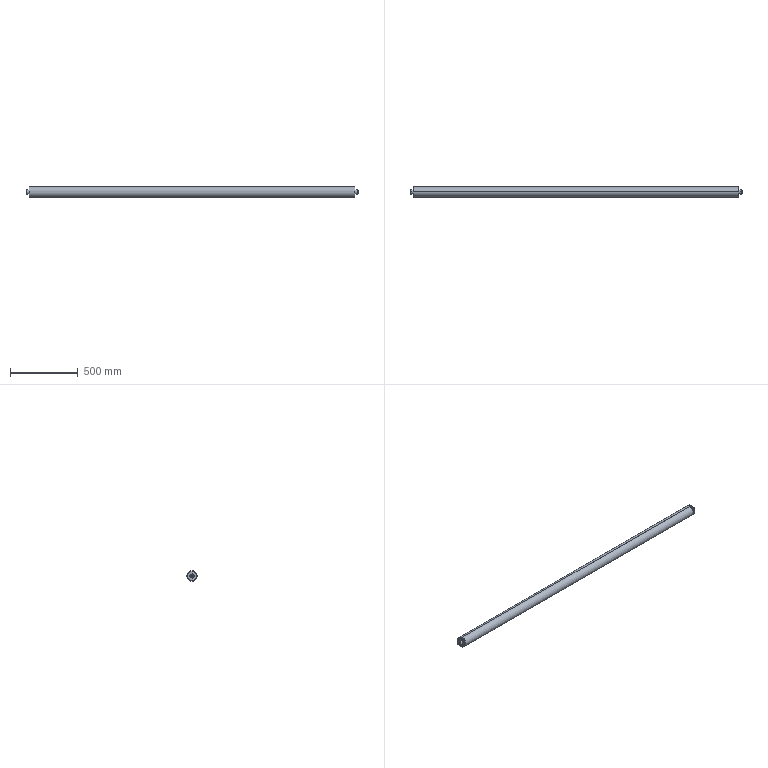Part | SolidWorks | features Chamfer 4, ICE 3, Revolution 3, 3DProfileFeature 1, HoleWzd 1, MirrorPattern 1 | 5 solids | 60 faces | box 2449 x 76 x 76 mm | volume 1229105 mm3 | cylinder 28 | plane 16 | cone 16 | commonest cylinder face diameters 30 x8 71.6 x6 8.5 x4 20 x4 5 x2 72 x2